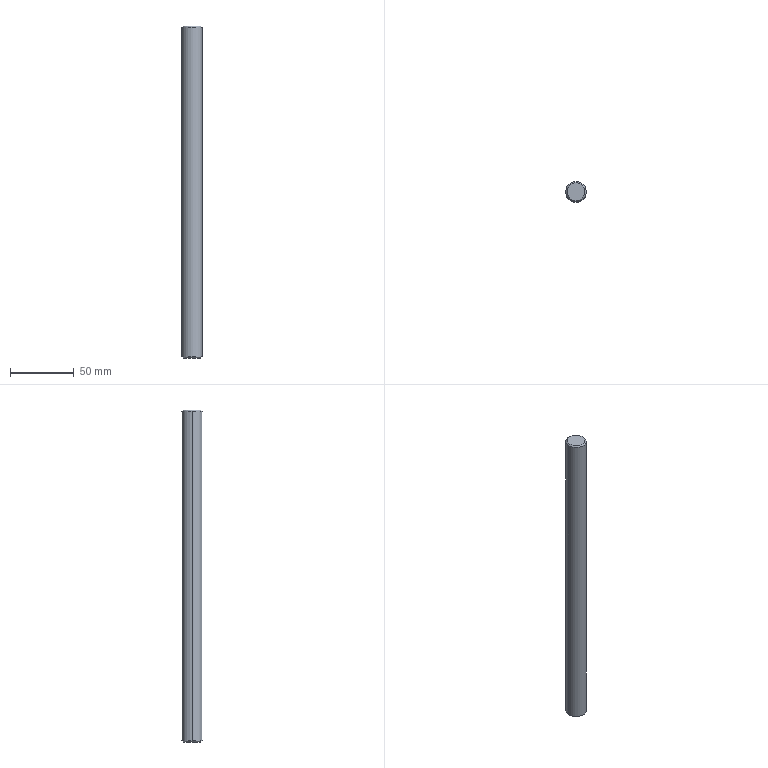Part | STEP file | fBY02F02M-00-21A | 1 solid | 8 faces | box 16 x 16 x 260 mm | volume 52228 mm3 | cone 4 | cylinder 2 | plane 2 | commonest cylinder face diameters 16 x2
STEP:
#1=CARTESIAN_POINT('',(0.,0.,0.));
#2=DIRECTION('',(0.,0.,1.));
#3=DIRECTION('',(1.,0.,0.));
#4=AXIS2_PLACEMENT_3D('',#1,#2,#3);
#5=CARTESIAN_POINT('',(-8.,0.,259.));
#6=VERTEX_POINT('',#5);
#7=CARTESIAN_POINT('',(8.,0.,259.));
#8=VERTEX_POINT('',#7);
#9=CARTESIAN_POINT('',(0.,0.,259.));
#10=DIRECTION('',(0.,0.,-1.));
#11=DIRECTION('',(-1.,0.,0.));
#12=AXIS2_PLACEMENT_3D('',#9,#10,#11);
#13=CIRCLE('',#12,8.);
#14=CARTESIAN_POINT('',(0.,0.,260.));
#15=DIRECTION('',(0.,0.,-1.));
#16=DIRECTION('',(-1.,0.,0.));
#17=AXIS2_PLACEMENT_3D('',#14,#15,#16);
#18=CYLINDRICAL_SURFACE('',#17,8.);
#19=CARTESIAN_POINT('',(0.,1.));
#20=DIRECTION('',(1.,0.));
#21=VECTOR('',#20,1.);
#22=LINE('',#19,#21);
#23=(GEOMETRIC_REPRESENTATION_CONTEXT(2)PARAMETRIC_REPRESENTATION_CONTEXT()REPRESENTATION_CONTEXT('',''));
#24=DEFINITIONAL_REPRESENTATION('',(#22),#23);
#25=PCURVE('',#18,#24);
#26=CARTESIAN_POINT('',(0.,0.,259.));
#27=DIRECTION('',(0.,0.,-1.));
#28=DIRECTION('',(-1.,0.,0.));
#29=AXIS2_PLACEMENT_3D('',#26,#27,#28);
#30=CONICAL_SURFACE('',#29,8.,0.7854);
#31=CARTESIAN_POINT('',(0.,0.));
#32=DIRECTION('',(1.,0.));
#33=VECTOR('',#32,1.);
#34=LINE('',#31,#33);
#35=(GEOMETRIC_REPRESENTATION_CONTEXT(2)PARAMETRIC_REPRESENTATION_CONTEXT()REPRESENTATION_CONTEXT('',''));
#36=DEFINITIONAL_REPRESENTATION('',(#34),#35);
#37=PCURVE('',#30,#36);
#38=SURFACE_CURVE('',#13,(#25,#37),.PCURVE_S1.);
#39=EDGE_CURVE('',#6,#8,#38,.T.);
#40=ORIENTED_EDGE('',*,*,#39,.T.);
#41=CARTESIAN_POINT('',(8.,0.,1.));
#42=VERTEX_POINT('',#41);
#43=CARTESIAN_POINT('',(8.,0.,260.));
#44=DIRECTION('',(0.,0.,-1.));
#45=VECTOR('',#44,1.);
#46=LINE('',#43,#45);
#47=CARTESIAN_POINT('',(3.142,0.));
#48=DIRECTION('',(0.,1.));
#49=VECTOR('',#48,1.);
#50=LINE('',#47,#49);
#51=(GEOMETRIC_REPRESENTATION_CONTEXT(2)PARAMETRIC_REPRESENTATION_CONTEXT()REPRESENTATION_CONTEXT('',''));
#52=DEFINITIONAL_REPRESENTATION('',(#50),#51);
#53=PCURVE('',#18,#52);
#54=CARTESIAN_POINT('',(0.,0.,260.));
#55=DIRECTION('',(0.,0.,-1.));
#56=DIRECTION('',(-1.,0.,0.));
#57=AXIS2_PLACEMENT_3D('',#54,#55,#56);
#58=CYLINDRICAL_SURFACE('',#57,8.);
#59=CARTESIAN_POINT('',(3.142,0.));
#60=DIRECTION('',(0.,1.));
#61=VECTOR('',#60,1.);
#62=LINE('',#59,#61);
#63=(GEOMETRIC_REPRESENTATION_CONTEXT(2)PARAMETRIC_REPRESENTATION_CONTEXT()REPRESENTATION_CONTEXT('',''));
#64=DEFINITIONAL_REPRESENTATION('',(#62),#63);
#65=PCURVE('',#58,#64);
#66=SURFACE_CURVE('',#46,(#53,#65),.PCURVE_S1.);
#67=EDGE_CURVE('',#8,#42,#66,.T.);
#68=ORIENTED_EDGE('',*,*,#67,.T.);
#69=CARTESIAN_POINT('',(-8.,0.,1.));
#70=VERTEX_POINT('',#69);
#71=CARTESIAN_POINT('',(0.,0.,1.));
#72=DIRECTION('',(0.,0.,1.));
#73=DIRECTION('',(-1.,0.,0.));
#74=AXIS2_PLACEMENT_3D('',#71,#72,#73);
#75=CIRCLE('',#74,8.);
#76=CARTESIAN_POINT('',(6.283,259.));
#77=DIRECTION('',(-1.,0.));
#78=VECTOR('',#77,1.);
#79=LINE('',#76,#78);
#80=(GEOMETRIC_REPRESENTATION_CONTEXT(2)PARAMETRIC_REPRESENTATION_CONTEXT()REPRESENTATION_CONTEXT('',''));
#81=DEFINITIONAL_REPRESENTATION('',(#79),#80);
#82=PCURVE('',#18,#81);
#83=CARTESIAN_POINT('',(0.,0.,1.));
#84=DIRECTION('',(0.,0.,1.));
#85=DIRECTION('',(1.,0.,0.));
#86=AXIS2_PLACEMENT_3D('',#83,#84,#85);
#87=CONICAL_SURFACE('',#86,8.,0.7854);
#88=CARTESIAN_POINT('',(-3.142,0.));
#89=DIRECTION('',(1.,0.));
#90=VECTOR('',#89,1.);
#91=LINE('',#88,#90);
#92=(GEOMETRIC_REPRESENTATION_CONTEXT(2)PARAMETRIC_REPRESENTATION_CONTEXT()REPRESENTATION_CONTEXT('',''));
#93=DEFINITIONAL_REPRESENTATION('',(#91),#92);
#94=PCURVE('',#87,#93);
#95=SURFACE_CURVE('',#75,(#82,#94),.PCURVE_S1.);
#96=EDGE_CURVE('',#42,#70,#95,.T.);
#97=ORIENTED_EDGE('',*,*,#96,.T.);
#98=CARTESIAN_POINT('',(-8.,0.,260.));
#99=DIRECTION('',(0.,0.,-1.));
#100=VECTOR('',#99,1.);
#101=LINE('',#98,#100);
#102=CARTESIAN_POINT('',(0.,0.));
#103=DIRECTION('',(0.,1.));
#104=VECTOR('',#103,1.);
#105=LINE('',#102,#104);
#106=(GEOMETRIC_REPRESENTATION_CONTEXT(2)PARAMETRIC_REPRESENTATION_CONTEXT()REPRESENTATION_CONTEXT('',''));
#107=DEFINITIONAL_REPRESENTATION('',(#105),#106);
#108=PCURVE('',#18,#107);
#109=CARTESIAN_POINT('',(6.283,0.));
#110=DIRECTION('',(0.,1.));
#111=VECTOR('',#110,1.);
#112=LINE('',#109,#111);
#113=(GEOMETRIC_REPRESENTATION_CONTEXT(2)PARAMETRIC_REPRESENTATION_CONTEXT()REPRESENTATION_CONTEXT('',''));
#114=DEFINITIONAL_REPRESENTATION('',(#112),#113);
#115=PCURVE('',#58,#114);
#116=SURFACE_CURVE('',#101,(#108,#115),.PCURVE_S1.);
#117=EDGE_CURVE('',#6,#70,#116,.T.);
#118=ORIENTED_EDGE('',*,*,#117,.F.);
#119=EDGE_LOOP('',(#40,#68,#97,#118));
#120=FACE_BOUND('',#119,.T.);
#121=ADVANCED_FACE('',(#120),#18,.T.);
#122=CARTESIAN_POINT('',(7.,0.,0.));
#123=VERTEX_POINT('',#122);
#124=CARTESIAN_POINT('',(-7.,0.,0.));
#125=VERTEX_POINT('',#124);
#126=CARTESIAN_POINT('',(0.,0.,0.));
#127=DIRECTION('',(0.,0.,1.));
#128=DIRECTION('',(1.,0.,0.));
#129=AXIS2_PLACEMENT_3D('',#126,#127,#128);
#130=CIRCLE('',#129,7.);
#131=CARTESIAN_POINT('',(0.,-1.));
#132=DIRECTION('',(1.,0.));
#133=VECTOR('',#132,1.);
#134=LINE('',#131,#133);
#135=(GEOMETRIC_REPRESENTATION_CONTEXT(2)PARAMETRIC_REPRESENTATION_CONTEXT()REPRESENTATION_CONTEXT('',''));
#136=DEFINITIONAL_REPRESENTATION('',(#134),#135);
#137=PCURVE('',#87,#136);
#138=CARTESIAN_POINT('',(0.,0.,0.));
#139=DIRECTION('',(0.,0.,1.));
#140=DIRECTION('',(1.,0.,0.));
#141=AXIS2_PLACEMENT_3D('',#138,#139,#140);
#142=PLANE('',#141);
#143=CARTESIAN_POINT('',(0.,0.));
#144=DIRECTION('',(1.,0.));
#145=AXIS2_PLACEMENT_2D('',#143,#144);
#146=CIRCLE('',#145,7.);
#147=(GEOMETRIC_REPRESENTATION_CONTEXT(2)PARAMETRIC_REPRESENTATION_CONTEXT()REPRESENTATION_CONTEXT('',''));
#148=DEFINITIONAL_REPRESENTATION('',(#146),#147);
#149=PCURVE('',#142,#148);
#150=SURFACE_CURVE('',#130,(#137,#149),.PCURVE_S1.);
#151=EDGE_CURVE('',#123,#125,#150,.T.);
#152=ORIENTED_EDGE('',*,*,#151,.T.);
#153=CARTESIAN_POINT('',(-8.,0.,1.));
#154=DIRECTION('',(-0.7071,0.,0.7071));
#155=VECTOR('',#154,1.);
#156=LINE('',#153,#155);
#157=CARTESIAN_POINT('',(3.142,0.));
#158=DIRECTION('',(0.,1.));
#159=VECTOR('',#158,1.);
#160=LINE('',#157,#159);
#161=(GEOMETRIC_REPRESENTATION_CONTEXT(2)PARAMETRIC_REPRESENTATION_CONTEXT()REPRESENTATION_CONTEXT('',''));
#162=DEFINITIONAL_REPRESENTATION('',(#160),#161);
#163=PCURVE('',#87,#162);
#164=CARTESIAN_POINT('',(0.,0.,1.));
#165=DIRECTION('',(0.,0.,1.));
#166=DIRECTION('',(1.,0.,0.));
#167=AXIS2_PLACEMENT_3D('',#164,#165,#166);
#168=CONICAL_SURFACE('',#167,8.,0.7854);
#169=CARTESIAN_POINT('',(3.142,0.));
#170=DIRECTION('',(0.,1.));
#171=VECTOR('',#170,1.);
#172=LINE('',#169,#171);
#173=(GEOMETRIC_REPRESENTATION_CONTEXT(2)PARAMETRIC_REPRESENTATION_CONTEXT()REPRESENTATION_CONTEXT('',''));
#174=DEFINITIONAL_REPRESENTATION('',(#172),#173);
#175=PCURVE('',#168,#174);
#176=SURFACE_CURVE('',#156,(#163,#175),.PCURVE_S1.);
#177=EDGE_CURVE('',#125,#70,#176,.T.);
#178=ORIENTED_EDGE('',*,*,#177,.T.);
#179=ORIENTED_EDGE('',*,*,#96,.F.);
#180=CARTESIAN_POINT('',(8.,0.,1.));
#181=DIRECTION('',(0.7071,0.,0.7071));
#182=VECTOR('',#181,1.);
#183=LINE('',#180,#182);
#184=CARTESIAN_POINT('',(0.,0.));
#185=DIRECTION('',(0.,1.));
#186=VECTOR('',#185,1.);
#187=LINE('',#184,#186);
#188=(GEOMETRIC_REPRESENTATION_CONTEXT(2)PARAMETRIC_REPRESENTATION_CONTEXT()REPRESENTATION_CONTEXT('',''));
#189=DEFINITIONAL_REPRESENTATION('',(#187),#188);
#190=PCURVE('',#87,#189);
#191=CARTESIAN_POINT('',(6.283,0.));
#192=DIRECTION('',(0.,1.));
#193=VECTOR('',#192,1.);
#194=LINE('',#191,#193);
#195=(GEOMETRIC_REPRESENTATION_CONTEXT(2)PARAMETRIC_REPRESENTATION_CONTEXT()REPRESENTATION_CONTEXT('',''));
#196=DEFINITIONAL_REPRESENTATION('',(#194),#195);
#197=PCURVE('',#168,#196);
#198=SURFACE_CURVE('',#183,(#190,#197),.PCURVE_S1.);
#199=EDGE_CURVE('',#123,#42,#198,.T.);
#200=ORIENTED_EDGE('',*,*,#199,.F.);
#201=EDGE_LOOP('',(#152,#178,#179,#200));
#202=FACE_BOUND('',#201,.T.);
#203=ADVANCED_FACE('',(#202),#87,.T.);
#204=CARTESIAN_POINT('',(-7.,0.,260.));
#205=VERTEX_POINT('',#204);
#206=CARTESIAN_POINT('',(7.,0.,260.));
#207=VERTEX_POINT('',#206);
#208=CARTESIAN_POINT('',(0.,0.,260.));
#209=DIRECTION('',(0.,0.,-1.));
#210=DIRECTION('',(-1.,0.,0.));
#211=AXIS2_PLACEMENT_3D('',#208,#209,#210);
#212=CIRCLE('',#211,7.);
#213=CARTESIAN_POINT('',(0.,-1.));
#214=DIRECTION('',(1.,0.));
#215=VECTOR('',#214,1.);
#216=LINE('',#213,#215);
#217=(GEOMETRIC_REPRESENTATION_CONTEXT(2)PARAMETRIC_REPRESENTATION_CONTEXT()REPRESENTATION_CONTEXT('',''));
#218=DEFINITIONAL_REPRESENTATION('',(#216),#217);
#219=PCURVE('',#30,#218);
#220=CARTESIAN_POINT('',(0.,0.,260.));
#221=DIRECTION('',(0.,0.,1.));
#222=DIRECTION('',(1.,0.,0.));
#223=AXIS2_PLACEMENT_3D('',#220,#221,#222);
#224=PLANE('',#223);
#225=CARTESIAN_POINT('',(-7.,0.));
#226=CARTESIAN_POINT('',(-7.,12.124));
#227=CARTESIAN_POINT('',(3.5,6.062));
#228=CARTESIAN_POINT('',(14.,0.));
#229=CARTESIAN_POINT('',(3.5,-6.062));
#230=CARTESIAN_POINT('',(-7.,-12.124));
#231=CARTESIAN_POINT('',(-7.,0.));
#232=(BOUNDED_CURVE()B_SPLINE_CURVE(2,(#225,#226,#227,#228,#229,#230,#231),.UNSPECIFIED.,.T.,.F.)B_SPLINE_CURVE_WITH_KNOTS((1,2,2,2,2,1),(-2.094,0.,2.094,4.189,6.283,8.378),.UNSPECIFIED.)CURVE()GEOMETRIC_REPRESENTATION_ITEM()RATIONAL_B_SPLINE_CURVE((1.,0.5,1.,0.5,1.,0.5,1.))REPRESENTATION_ITEM(''));
#233=(GEOMETRIC_REPRESENTATION_CONTEXT(2)PARAMETRIC_REPRESENTATION_CONTEXT()REPRESENTATION_CONTEXT('',''));
#234=DEFINITIONAL_REPRESENTATION('',(#232),#233);
#235=PCURVE('',#224,#234);
#236=SURFACE_CURVE('',#212,(#219,#235),.PCURVE_S1.);
#237=EDGE_CURVE('',#205,#207,#236,.T.);
#238=ORIENTED_EDGE('',*,*,#237,.T.);
#239=CARTESIAN_POINT('',(8.,0.,259.));
#240=DIRECTION('',(0.7071,0.,-0.7071));
#241=VECTOR('',#240,1.);
#242=LINE('',#239,#241);
#243=CARTESIAN_POINT('',(3.142,0.));
#244=DIRECTION('',(0.,1.));
#245=VECTOR('',#244,1.);
#246=LINE('',#243,#245);
#247=(GEOMETRIC_REPRESENTATION_CONTEXT(2)PARAMETRIC_REPRESENTATION_CONTEXT()REPRESENTATION_CONTEXT('',''));
#248=DEFINITIONAL_REPRESENTATION('',(#246),#247);
#249=PCURVE('',#30,#248);
#250=CARTESIAN_POINT('',(0.,0.,259.));
#251=DIRECTION('',(0.,0.,-1.));
#252=DIRECTION('',(-1.,0.,0.));
#253=AXIS2_PLACEMENT_3D('',#250,#251,#252);
#254=CONICAL_SURFACE('',#253,8.,0.7854);
#255=CARTESIAN_POINT('',(3.142,0.));
#256=DIRECTION('',(0.,1.));
#257=VECTOR('',#256,1.);
#258=LINE('',#255,#257);
#259=(GEOMETRIC_REPRESENTATION_CONTEXT(2)PARAMETRIC_REPRESENTATION_CONTEXT()REPRESENTATION_CONTEXT('',''));
#260=DEFINITIONAL_REPRESENTATION('',(#258),#259);
#261=PCURVE('',#254,#260);
#262=SURFACE_CURVE('',#242,(#249,#261),.PCURVE_S1.);
#263=EDGE_CURVE('',#207,#8,#262,.T.);
#264=ORIENTED_EDGE('',*,*,#263,.T.);
#265=ORIENTED_EDGE('',*,*,#39,.F.);
#266=CARTESIAN_POINT('',(-8.,0.,259.));
#267=DIRECTION('',(-0.7071,0.,-0.7071));
#268=VECTOR('',#267,1.);
#269=LINE('',#266,#268);
#270=CARTESIAN_POINT('',(0.,0.));
#271=DIRECTION('',(0.,1.));
#272=VECTOR('',#271,1.);
#273=LINE('',#270,#272);
#274=(GEOMETRIC_REPRESENTATION_CONTEXT(2)PARAMETRIC_REPRESENTATION_CONTEXT()REPRESENTATION_CONTEXT('',''));
#275=DEFINITIONAL_REPRESENTATION('',(#273),#274);
#276=PCURVE('',#30,#275);
#277=CARTESIAN_POINT('',(6.283,0.));
#278=DIRECTION('',(0.,1.));
#279=VECTOR('',#278,1.);
#280=LINE('',#277,#279);
#281=(GEOMETRIC_REPRESENTATION_CONTEXT(2)PARAMETRIC_REPRESENTATION_CONTEXT()REPRESENTATION_CONTEXT('',''));
#282=DEFINITIONAL_REPRESENTATION('',(#280),#281);
#283=PCURVE('',#254,#282);
#284=SURFACE_CURVE('',#269,(#276,#283),.PCURVE_S1.);
#285=EDGE_CURVE('',#205,#6,#284,.T.);
#286=ORIENTED_EDGE('',*,*,#285,.F.);
#287=EDGE_LOOP('',(#238,#264,#265,#286));
#288=FACE_BOUND('',#287,.T.);
#289=ADVANCED_FACE('',(#288),#30,.T.);
#290=ORIENTED_EDGE('',*,*,#67,.F.);
#291=CARTESIAN_POINT('',(0.,0.,259.));
#292=DIRECTION('',(0.,0.,-1.));
#293=DIRECTION('',(-1.,0.,0.));
#294=AXIS2_PLACEMENT_3D('',#291,#292,#293);
#295=CIRCLE('',#294,8.);
#296=CARTESIAN_POINT('',(0.,1.));
#297=DIRECTION('',(1.,0.));
#298=VECTOR('',#297,1.);
#299=LINE('',#296,#298);
#300=(GEOMETRIC_REPRESENTATION_CONTEXT(2)PARAMETRIC_REPRESENTATION_CONTEXT()REPRESENTATION_CONTEXT('',''));
#301=DEFINITIONAL_REPRESENTATION('',(#299),#300);
#302=PCURVE('',#58,#301);
#303=CARTESIAN_POINT('',(0.,0.));
#304=DIRECTION('',(1.,0.));
#305=VECTOR('',#304,1.);
#306=LINE('',#303,#305);
#307=(GEOMETRIC_REPRESENTATION_CONTEXT(2)PARAMETRIC_REPRESENTATION_CONTEXT()REPRESENTATION_CONTEXT('',''));
#308=DEFINITIONAL_REPRESENTATION('',(#306),#307);
#309=PCURVE('',#254,#308);
#310=SURFACE_CURVE('',#295,(#302,#309),.PCURVE_S1.);
#311=EDGE_CURVE('',#8,#6,#310,.T.);
#312=ORIENTED_EDGE('',*,*,#311,.T.);
#313=ORIENTED_EDGE('',*,*,#117,.T.);
#314=CARTESIAN_POINT('',(0.,0.,1.));
#315=DIRECTION('',(0.,0.,1.));
#316=DIRECTION('',(-1.,0.,0.));
#317=AXIS2_PLACEMENT_3D('',#314,#315,#316);
#318=CIRCLE('',#317,8.);
#319=CARTESIAN_POINT('',(6.283,259.));
#320=DIRECTION('',(-1.,0.));
#321=VECTOR('',#320,1.);
#322=LINE('',#319,#321);
#323=(GEOMETRIC_REPRESENTATION_CONTEXT(2)PARAMETRIC_REPRESENTATION_CONTEXT()REPRESENTATION_CONTEXT('',''));
#324=DEFINITIONAL_REPRESENTATION('',(#322),#323);
#325=PCURVE('',#58,#324);
#326=CARTESIAN_POINT('',(3.142,0.));
#327=DIRECTION('',(1.,0.));
#328=VECTOR('',#327,1.);
#329=LINE('',#326,#328);
#330=(GEOMETRIC_REPRESENTATION_CONTEXT(2)PARAMETRIC_REPRESENTATION_CONTEXT()REPRESENTATION_CONTEXT('',''));
#331=DEFINITIONAL_REPRESENTATION('',(#329),#330);
#332=PCURVE('',#168,#331);
#333=SURFACE_CURVE('',#318,(#325,#332),.PCURVE_S1.);
#334=EDGE_CURVE('',#70,#42,#333,.T.);
#335=ORIENTED_EDGE('',*,*,#334,.T.);
#336=EDGE_LOOP('',(#290,#312,#313,#335));
#337=FACE_BOUND('',#336,.T.);
#338=ADVANCED_FACE('',(#337),#58,.T.);
#339=ORIENTED_EDGE('',*,*,#177,.F.);
#340=CARTESIAN_POINT('',(0.,0.,0.));
#341=DIRECTION('',(0.,0.,1.));
#342=DIRECTION('',(1.,0.,0.));
#343=AXIS2_PLACEMENT_3D('',#340,#341,#342);
#344=CIRCLE('',#343,7.);
#345=CARTESIAN_POINT('',(0.,-1.));
#346=DIRECTION('',(1.,0.));
#347=VECTOR('',#346,1.);
#348=LINE('',#345,#347);
#349=(GEOMETRIC_REPRESENTATION_CONTEXT(2)PARAMETRIC_REPRESENTATION_CONTEXT()REPRESENTATION_CONTEXT('',''));
#350=DEFINITIONAL_REPRESENTATION('',(#348),#349);
#351=PCURVE('',#168,#350);
#352=CARTESIAN_POINT('',(0.,0.));
#353=DIRECTION('',(1.,0.));
#354=AXIS2_PLACEMENT_2D('',#352,#353);
#355=CIRCLE('',#354,7.);
#356=(GEOMETRIC_REPRESENTATION_CONTEXT(2)PARAMETRIC_REPRESENTATION_CONTEXT()REPRESENTATION_CONTEXT('',''));
#357=DEFINITIONAL_REPRESENTATION('',(#355),#356);
#358=PCURVE('',#142,#357);
#359=SURFACE_CURVE('',#344,(#351,#358),.PCURVE_S1.);
#360=EDGE_CURVE('',#125,#123,#359,.T.);
#361=ORIENTED_EDGE('',*,*,#360,.T.);
#362=ORIENTED_EDGE('',*,*,#199,.T.);
#363=ORIENTED_EDGE('',*,*,#334,.F.);
#364=EDGE_LOOP('',(#339,#361,#362,#363));
#365=FACE_BOUND('',#364,.T.);
#366=ADVANCED_FACE('',(#365),#168,.T.);
#367=ORIENTED_EDGE('',*,*,#263,.F.);
#368=CARTESIAN_POINT('',(0.,0.,260.));
#369=DIRECTION('',(0.,0.,-1.));
#370=DIRECTION('',(-1.,0.,0.));
#371=AXIS2_PLACEMENT_3D('',#368,#369,#370);
#372=CIRCLE('',#371,7.);
#373=CARTESIAN_POINT('',(0.,-1.));
#374=DIRECTION('',(1.,0.));
#375=VECTOR('',#374,1.);
#376=LINE('',#373,#375);
#377=(GEOMETRIC_REPRESENTATION_CONTEXT(2)PARAMETRIC_REPRESENTATION_CONTEXT()REPRESENTATION_CONTEXT('',''));
#378=DEFINITIONAL_REPRESENTATION('',(#376),#377);
#379=PCURVE('',#254,#378);
#380=CARTESIAN_POINT('',(-7.,0.));
#381=CARTESIAN_POINT('',(-7.,12.124));
#382=CARTESIAN_POINT('',(3.5,6.062));
#383=CARTESIAN_POINT('',(14.,0.));
#384=CARTESIAN_POINT('',(3.5,-6.062));
#385=CARTESIAN_POINT('',(-7.,-12.124));
#386=CARTESIAN_POINT('',(-7.,0.));
#387=(BOUNDED_CURVE()B_SPLINE_CURVE(2,(#380,#381,#382,#383,#384,#385,#386),.UNSPECIFIED.,.T.,.F.)B_SPLINE_CURVE_WITH_KNOTS((1,2,2,2,2,1),(-2.094,0.,2.094,4.189,6.283,8.378),.UNSPECIFIED.)CURVE()GEOMETRIC_REPRESENTATION_ITEM()RATIONAL_B_SPLINE_CURVE((1.,0.5,1.,0.5,1.,0.5,1.))REPRESENTATION_ITEM(''));
#388=(GEOMETRIC_REPRESENTATION_CONTEXT(2)PARAMETRIC_REPRESENTATION_CONTEXT()REPRESENTATION_CONTEXT('',''));
#389=DEFINITIONAL_REPRESENTATION('',(#387),#388);
#390=PCURVE('',#224,#389);
#391=SURFACE_CURVE('',#372,(#379,#390),.PCURVE_S1.);
#392=EDGE_CURVE('',#207,#205,#391,.T.);
#393=ORIENTED_EDGE('',*,*,#392,.T.);
#394=ORIENTED_EDGE('',*,*,#285,.T.);
#395=ORIENTED_EDGE('',*,*,#311,.F.);
#396=EDGE_LOOP('',(#367,#393,#394,#395));
#397=FACE_BOUND('',#396,.T.);
#398=ADVANCED_FACE('',(#397),#254,.T.);
#399=ORIENTED_EDGE('',*,*,#151,.F.);
#400=ORIENTED_EDGE('',*,*,#360,.F.);
#401=EDGE_LOOP('',(#399,#400));
#402=FACE_BOUND('',#401,.T.);
#403=ADVANCED_FACE('',(#402),#142,.F.);
#404=ORIENTED_EDGE('',*,*,#237,.F.);
#405=ORIENTED_EDGE('',*,*,#392,.F.);
#406=EDGE_LOOP('',(#404,#405));
#407=FACE_BOUND('',#406,.T.);
#408=ADVANCED_FACE('',(#407),#224,.T.);
#409=CLOSED_SHELL('',(#121,#203,#289,#338,#366,#398,#403,#408));
#410=MANIFOLD_SOLID_BREP('',#409);
#411=(LENGTH_UNIT()NAMED_UNIT(*)SI_UNIT(.MILLI.,.METRE.));
#412=UNCERTAINTY_MEASURE_WITH_UNIT(LENGTH_MEASURE(0.0000001),#411,'','');
#413=(NAMED_UNIT(*)PLANE_ANGLE_UNIT()SI_UNIT($,.RADIAN.));
#414=(NAMED_UNIT(*)SI_UNIT($,.STERADIAN.)SOLID_ANGLE_UNIT());
#415=(GEOMETRIC_REPRESENTATION_CONTEXT(3)GLOBAL_UNCERTAINTY_ASSIGNED_CONTEXT((#412))GLOBAL_UNIT_ASSIGNED_CONTEXT((#411,#413,#414))REPRESENTATION_CONTEXT('',''));
#416=ADVANCED_BREP_SHAPE_REPRESENTATION('',(#4,#410),#415);